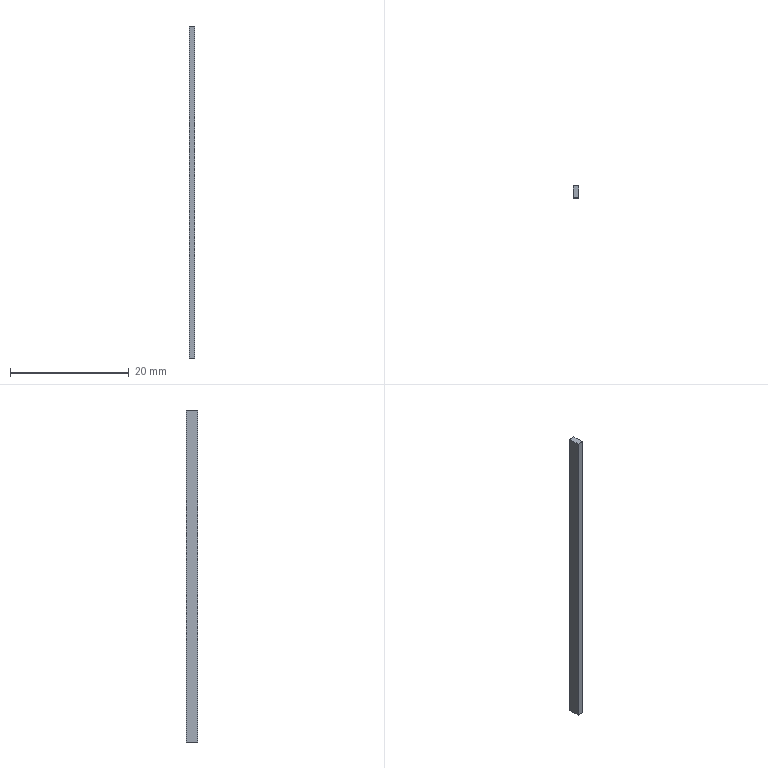Part | NX | features BREP 2 | 2 solids | 12 faces | box 1 x 2 x 56 mm | volume 224 mm3 | plane 12
STEP:
#1=CARTESIAN_POINT('',(0.5,-1.,-4.));
#2=VERTEX_POINT('',#1);
#3=CARTESIAN_POINT('',(0.5,-1.,52.));
#4=VERTEX_POINT('',#3);
#5=CARTESIAN_POINT('',(0.5,-1.,0.));
#6=DIRECTION('',(0.,0.,1.));
#7=VECTOR('',#6,1000.);
#8=LINE('',#5,#7);
#9=EDGE_CURVE('',#2,#4,#8,.T.);
#10=ORIENTED_EDGE('',*,*,#9,.T.);
#11=CARTESIAN_POINT('',(-0.5,-1.,52.));
#12=VERTEX_POINT('',#11);
#13=CARTESIAN_POINT('',(-3.542,-1.,52.));
#14=DIRECTION('',(1.,0.,0.));
#15=VECTOR('',#14,1000.);
#16=LINE('',#13,#15);
#17=EDGE_CURVE('',#12,#4,#16,.T.);
#18=ORIENTED_EDGE('',*,*,#17,.F.);
#19=CARTESIAN_POINT('',(-0.5,-1.,-4.));
#20=VERTEX_POINT('',#19);
#21=CARTESIAN_POINT('',(-0.5,-1.,0.));
#22=DIRECTION('',(0.,0.,1.));
#23=VECTOR('',#22,1000.);
#24=LINE('',#21,#23);
#25=EDGE_CURVE('',#20,#12,#24,.T.);
#26=ORIENTED_EDGE('',*,*,#25,.F.);
#27=CARTESIAN_POINT('',(-3.542,-1.,-4.));
#28=DIRECTION('',(1.,0.,0.));
#29=VECTOR('',#28,1000.);
#30=LINE('',#27,#29);
#31=EDGE_CURVE('',#20,#2,#30,.T.);
#32=ORIENTED_EDGE('',*,*,#31,.T.);
#33=EDGE_LOOP('',(#10,#18,#26,#32));
#34=FACE_BOUND('',#33,.T.);
#35=CARTESIAN_POINT('',(-3.542,-1.,0.));
#36=DIRECTION('',(0.,-1.,0.));
#37=DIRECTION('',(-1.,0.,0.));
#38=AXIS2_PLACEMENT_3D('',#35,#36,#37);
#39=PLANE('',#38);
#40=ADVANCED_FACE('',(#34),#39,.T.);
#41=ORIENTED_EDGE('',*,*,#25,.T.);
#42=CARTESIAN_POINT('',(-0.5,1.,52.));
#43=VERTEX_POINT('',#42);
#44=CARTESIAN_POINT('',(-0.5,-13.298,52.));
#45=DIRECTION('',(0.,-1.,0.));
#46=VECTOR('',#45,1000.);
#47=LINE('',#44,#46);
#48=EDGE_CURVE('',#43,#12,#47,.T.);
#49=ORIENTED_EDGE('',*,*,#48,.F.);
#50=CARTESIAN_POINT('',(-0.5,1.,-4.));
#51=VERTEX_POINT('',#50);
#52=CARTESIAN_POINT('',(-0.5,1.,0.));
#53=DIRECTION('',(0.,0.,1.));
#54=VECTOR('',#53,1000.);
#55=LINE('',#52,#54);
#56=EDGE_CURVE('',#51,#43,#55,.T.);
#57=ORIENTED_EDGE('',*,*,#56,.F.);
#58=CARTESIAN_POINT('',(-0.5,-13.298,-4.));
#59=DIRECTION('',(0.,-1.,0.));
#60=VECTOR('',#59,1000.);
#61=LINE('',#58,#60);
#62=EDGE_CURVE('',#51,#20,#61,.T.);
#63=ORIENTED_EDGE('',*,*,#62,.T.);
#64=EDGE_LOOP('',(#41,#49,#57,#63));
#65=FACE_BOUND('',#64,.T.);
#66=CARTESIAN_POINT('',(-0.5,-1.593,0.));
#67=DIRECTION('',(1.,0.,0.));
#68=DIRECTION('',(0.,-1.,0.));
#69=AXIS2_PLACEMENT_3D('',#66,#67,#68);
#70=PLANE('',#69);
#71=ADVANCED_FACE('',(#65),#70,.F.);
#72=ORIENTED_EDGE('',*,*,#56,.T.);
#73=CARTESIAN_POINT('',(0.5,1.,52.));
#74=VERTEX_POINT('',#73);
#75=CARTESIAN_POINT('',(-3.542,1.,52.));
#76=DIRECTION('',(-1.,0.,0.));
#77=VECTOR('',#76,1000.);
#78=LINE('',#75,#77);
#79=EDGE_CURVE('',#74,#43,#78,.T.);
#80=ORIENTED_EDGE('',*,*,#79,.F.);
#81=CARTESIAN_POINT('',(0.5,1.,-4.));
#82=VERTEX_POINT('',#81);
#83=CARTESIAN_POINT('',(0.5,1.,0.));
#84=DIRECTION('',(0.,0.,1.));
#85=VECTOR('',#84,1000.);
#86=LINE('',#83,#85);
#87=EDGE_CURVE('',#82,#74,#86,.T.);
#88=ORIENTED_EDGE('',*,*,#87,.F.);
#89=CARTESIAN_POINT('',(-3.542,1.,-4.));
#90=DIRECTION('',(-1.,0.,0.));
#91=VECTOR('',#90,1000.);
#92=LINE('',#89,#91);
#93=EDGE_CURVE('',#82,#51,#92,.T.);
#94=ORIENTED_EDGE('',*,*,#93,.T.);
#95=EDGE_LOOP('',(#72,#80,#88,#94));
#96=FACE_BOUND('',#95,.T.);
#97=CARTESIAN_POINT('',(-3.542,1.,0.));
#98=DIRECTION('',(0.,-1.,0.));
#99=DIRECTION('',(-1.,0.,0.));
#100=AXIS2_PLACEMENT_3D('',#97,#98,#99);
#101=PLANE('',#100);
#102=ADVANCED_FACE('',(#96),#101,.F.);
#103=CARTESIAN_POINT('',(0.5,-13.298,-4.));
#104=DIRECTION('',(0.,1.,0.));
#105=VECTOR('',#104,1000.);
#106=LINE('',#103,#105);
#107=EDGE_CURVE('',#2,#82,#106,.T.);
#108=ORIENTED_EDGE('',*,*,#107,.T.);
#109=ORIENTED_EDGE('',*,*,#87,.T.);
#110=CARTESIAN_POINT('',(0.5,-13.298,52.));
#111=DIRECTION('',(0.,1.,0.));
#112=VECTOR('',#111,1000.);
#113=LINE('',#110,#112);
#114=EDGE_CURVE('',#4,#74,#113,.T.);
#115=ORIENTED_EDGE('',*,*,#114,.F.);
#116=ORIENTED_EDGE('',*,*,#9,.F.);
#117=EDGE_LOOP('',(#108,#109,#115,#116));
#118=FACE_BOUND('',#117,.T.);
#119=CARTESIAN_POINT('',(0.5,4.,0.));
#120=DIRECTION('',(-1.,0.,0.));
#121=DIRECTION('',(0.,1.,0.));
#122=AXIS2_PLACEMENT_3D('',#119,#120,#121);
#123=PLANE('',#122);
#124=ADVANCED_FACE('',(#118),#123,.F.);
#125=ORIENTED_EDGE('',*,*,#79,.T.);
#126=ORIENTED_EDGE('',*,*,#48,.T.);
#127=ORIENTED_EDGE('',*,*,#17,.T.);
#128=ORIENTED_EDGE('',*,*,#114,.T.);
#129=EDGE_LOOP('',(#125,#126,#127,#128));
#130=FACE_BOUND('',#129,.T.);
#131=CARTESIAN_POINT('',(-3.542,-13.298,52.));
#132=DIRECTION('',(0.,0.,1.));
#133=DIRECTION('',(-1.,0.,0.));
#134=AXIS2_PLACEMENT_3D('',#131,#132,#133);
#135=PLANE('',#134);
#136=ADVANCED_FACE('',(#130),#135,.T.);
#137=ORIENTED_EDGE('',*,*,#93,.F.);
#138=ORIENTED_EDGE('',*,*,#107,.F.);
#139=ORIENTED_EDGE('',*,*,#31,.F.);
#140=ORIENTED_EDGE('',*,*,#62,.F.);
#141=EDGE_LOOP('',(#137,#138,#139,#140));
#142=FACE_BOUND('',#141,.T.);
#143=CARTESIAN_POINT('',(-3.542,-13.298,-4.));
#144=DIRECTION('',(0.,0.,1.));
#145=DIRECTION('',(-1.,0.,0.));
#146=AXIS2_PLACEMENT_3D('',#143,#144,#145);
#147=PLANE('',#146);
#148=ADVANCED_FACE('',(#142),#147,.F.);
#149=CLOSED_SHELL('',(#40,#71,#102,#124,#136,#148));
#150=MANIFOLD_SOLID_BREP('',#149);
#151=CARTESIAN_POINT('',(0.5,-1.,-4.));
#152=VERTEX_POINT('',#151);
#153=CARTESIAN_POINT('',(0.5,-1.,52.));
#154=VERTEX_POINT('',#153);
#155=CARTESIAN_POINT('',(0.5,-1.,0.));
#156=DIRECTION('',(0.,0.,1.));
#157=VECTOR('',#156,1000.);
#158=LINE('',#155,#157);
#159=EDGE_CURVE('',#152,#154,#158,.T.);
#160=ORIENTED_EDGE('',*,*,#159,.T.);
#161=CARTESIAN_POINT('',(-0.5,-1.,52.));
#162=VERTEX_POINT('',#161);
#163=CARTESIAN_POINT('',(-3.542,-1.,52.));
#164=DIRECTION('',(1.,0.,0.));
#165=VECTOR('',#164,1000.);
#166=LINE('',#163,#165);
#167=EDGE_CURVE('',#162,#154,#166,.T.);
#168=ORIENTED_EDGE('',*,*,#167,.F.);
#169=CARTESIAN_POINT('',(-0.5,-1.,-4.));
#170=VERTEX_POINT('',#169);
#171=CARTESIAN_POINT('',(-0.5,-1.,0.));
#172=DIRECTION('',(0.,0.,1.));
#173=VECTOR('',#172,1000.);
#174=LINE('',#171,#173);
#175=EDGE_CURVE('',#170,#162,#174,.T.);
#176=ORIENTED_EDGE('',*,*,#175,.F.);
#177=CARTESIAN_POINT('',(-3.542,-1.,-4.));
#178=DIRECTION('',(1.,0.,0.));
#179=VECTOR('',#178,1000.);
#180=LINE('',#177,#179);
#181=EDGE_CURVE('',#170,#152,#180,.T.);
#182=ORIENTED_EDGE('',*,*,#181,.T.);
#183=EDGE_LOOP('',(#160,#168,#176,#182));
#184=FACE_BOUND('',#183,.T.);
#185=CARTESIAN_POINT('',(-3.542,-1.,0.));
#186=DIRECTION('',(0.,-1.,0.));
#187=DIRECTION('',(-1.,0.,0.));
#188=AXIS2_PLACEMENT_3D('',#185,#186,#187);
#189=PLANE('',#188);
#190=ADVANCED_FACE('',(#184),#189,.T.);
#191=ORIENTED_EDGE('',*,*,#175,.T.);
#192=CARTESIAN_POINT('',(-0.5,1.,52.));
#193=VERTEX_POINT('',#192);
#194=CARTESIAN_POINT('',(-0.5,-13.298,52.));
#195=DIRECTION('',(0.,-1.,0.));
#196=VECTOR('',#195,1000.);
#197=LINE('',#194,#196);
#198=EDGE_CURVE('',#193,#162,#197,.T.);
#199=ORIENTED_EDGE('',*,*,#198,.F.);
#200=CARTESIAN_POINT('',(-0.5,1.,-4.));
#201=VERTEX_POINT('',#200);
#202=CARTESIAN_POINT('',(-0.5,1.,0.));
#203=DIRECTION('',(0.,0.,1.));
#204=VECTOR('',#203,1000.);
#205=LINE('',#202,#204);
#206=EDGE_CURVE('',#201,#193,#205,.T.);
#207=ORIENTED_EDGE('',*,*,#206,.F.);
#208=CARTESIAN_POINT('',(-0.5,-13.298,-4.));
#209=DIRECTION('',(0.,-1.,0.));
#210=VECTOR('',#209,1000.);
#211=LINE('',#208,#210);
#212=EDGE_CURVE('',#201,#170,#211,.T.);
#213=ORIENTED_EDGE('',*,*,#212,.T.);
#214=EDGE_LOOP('',(#191,#199,#207,#213));
#215=FACE_BOUND('',#214,.T.);
#216=CARTESIAN_POINT('',(-0.5,-1.593,0.));
#217=DIRECTION('',(1.,0.,0.));
#218=DIRECTION('',(0.,-1.,0.));
#219=AXIS2_PLACEMENT_3D('',#216,#217,#218);
#220=PLANE('',#219);
#221=ADVANCED_FACE('',(#215),#220,.F.);
#222=ORIENTED_EDGE('',*,*,#206,.T.);
#223=CARTESIAN_POINT('',(0.5,1.,52.));
#224=VERTEX_POINT('',#223);
#225=CARTESIAN_POINT('',(-3.542,1.,52.));
#226=DIRECTION('',(-1.,0.,0.));
#227=VECTOR('',#226,1000.);
#228=LINE('',#225,#227);
#229=EDGE_CURVE('',#224,#193,#228,.T.);
#230=ORIENTED_EDGE('',*,*,#229,.F.);
#231=CARTESIAN_POINT('',(0.5,1.,-4.));
#232=VERTEX_POINT('',#231);
#233=CARTESIAN_POINT('',(0.5,1.,0.));
#234=DIRECTION('',(0.,0.,1.));
#235=VECTOR('',#234,1000.);
#236=LINE('',#233,#235);
#237=EDGE_CURVE('',#232,#224,#236,.T.);
#238=ORIENTED_EDGE('',*,*,#237,.F.);
#239=CARTESIAN_POINT('',(-3.542,1.,-4.));
#240=DIRECTION('',(-1.,0.,0.));
#241=VECTOR('',#240,1000.);
#242=LINE('',#239,#241);
#243=EDGE_CURVE('',#232,#201,#242,.T.);
#244=ORIENTED_EDGE('',*,*,#243,.T.);
#245=EDGE_LOOP('',(#222,#230,#238,#244));
#246=FACE_BOUND('',#245,.T.);
#247=CARTESIAN_POINT('',(-3.542,1.,0.));
#248=DIRECTION('',(0.,-1.,0.));
#249=DIRECTION('',(-1.,0.,0.));
#250=AXIS2_PLACEMENT_3D('',#247,#248,#249);
#251=PLANE('',#250);
#252=ADVANCED_FACE('',(#246),#251,.F.);
#253=CARTESIAN_POINT('',(0.5,-13.298,-4.));
#254=DIRECTION('',(0.,1.,0.));
#255=VECTOR('',#254,1000.);
#256=LINE('',#253,#255);
#257=EDGE_CURVE('',#152,#232,#256,.T.);
#258=ORIENTED_EDGE('',*,*,#257,.T.);
#259=ORIENTED_EDGE('',*,*,#237,.T.);
#260=CARTESIAN_POINT('',(0.5,-13.298,52.));
#261=DIRECTION('',(0.,1.,0.));
#262=VECTOR('',#261,1000.);
#263=LINE('',#260,#262);
#264=EDGE_CURVE('',#154,#224,#263,.T.);
#265=ORIENTED_EDGE('',*,*,#264,.F.);
#266=ORIENTED_EDGE('',*,*,#159,.F.);
#267=EDGE_LOOP('',(#258,#259,#265,#266));
#268=FACE_BOUND('',#267,.T.);
#269=CARTESIAN_POINT('',(0.5,4.,0.));
#270=DIRECTION('',(-1.,0.,0.));
#271=DIRECTION('',(0.,1.,0.));
#272=AXIS2_PLACEMENT_3D('',#269,#270,#271);
#273=PLANE('',#272);
#274=ADVANCED_FACE('',(#268),#273,.F.);
#275=ORIENTED_EDGE('',*,*,#229,.T.);
#276=ORIENTED_EDGE('',*,*,#198,.T.);
#277=ORIENTED_EDGE('',*,*,#167,.T.);
#278=ORIENTED_EDGE('',*,*,#264,.T.);
#279=EDGE_LOOP('',(#275,#276,#277,#278));
#280=FACE_BOUND('',#279,.T.);
#281=CARTESIAN_POINT('',(-3.542,-13.298,52.));
#282=DIRECTION('',(0.,0.,1.));
#283=DIRECTION('',(-1.,0.,0.));
#284=AXIS2_PLACEMENT_3D('',#281,#282,#283);
#285=PLANE('',#284);
#286=ADVANCED_FACE('',(#280),#285,.T.);
#287=ORIENTED_EDGE('',*,*,#243,.F.);
#288=ORIENTED_EDGE('',*,*,#257,.F.);
#289=ORIENTED_EDGE('',*,*,#181,.F.);
#290=ORIENTED_EDGE('',*,*,#212,.F.);
#291=EDGE_LOOP('',(#287,#288,#289,#290));
#292=FACE_BOUND('',#291,.T.);
#293=CARTESIAN_POINT('',(-3.542,-13.298,-4.));
#294=DIRECTION('',(0.,0.,1.));
#295=DIRECTION('',(-1.,0.,0.));
#296=AXIS2_PLACEMENT_3D('',#293,#294,#295);
#297=PLANE('',#296);
#298=ADVANCED_FACE('',(#292),#297,.F.);
#299=CLOSED_SHELL('',(#190,#221,#252,#274,#286,#298));
#300=MANIFOLD_SOLID_BREP('',#299);
#301=(LENGTH_UNIT()NAMED_UNIT(*)SI_UNIT(.MILLI.,.METRE.));
#302=UNCERTAINTY_MEASURE_WITH_UNIT(LENGTH_MEASURE(0.00001),#301,'','');
#303=(NAMED_UNIT(*)PLANE_ANGLE_UNIT()SI_UNIT($,.RADIAN.));
#304=(NAMED_UNIT(*)SI_UNIT($,.STERADIAN.)SOLID_ANGLE_UNIT());
#305=(GEOMETRIC_REPRESENTATION_CONTEXT(3)GLOBAL_UNCERTAINTY_ASSIGNED_CONTEXT((#302))GLOBAL_UNIT_ASSIGNED_CONTEXT((#301,#303,#304))REPRESENTATION_CONTEXT('',''));
#306=ADVANCED_BREP_SHAPE_REPRESENTATION('',(#150,#300),#305);